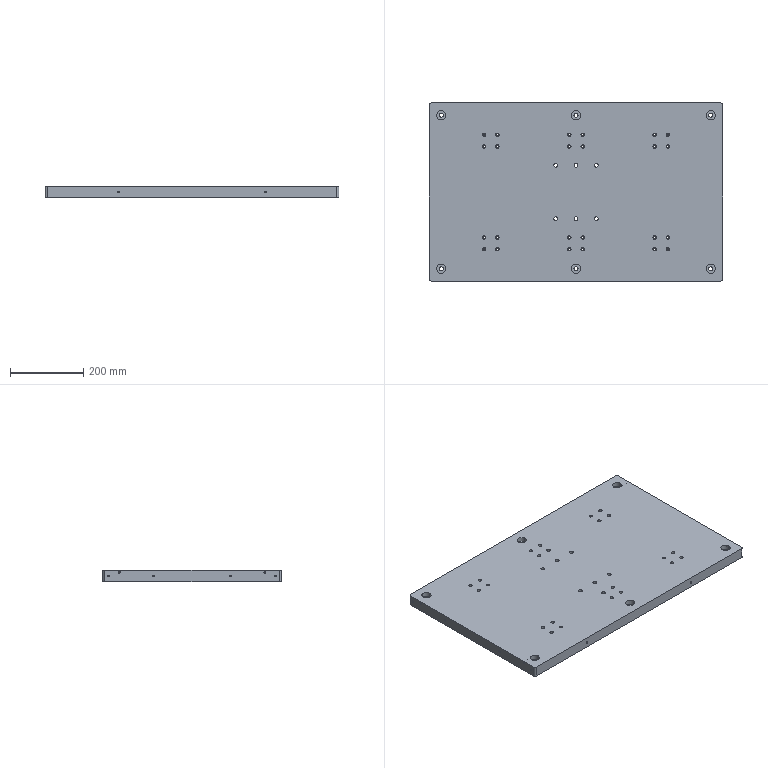Part | 1 solid | 238 faces | box 800 x 485 x 30 mm | volume 11530957 mm3 | cylinder 180 | plane 58 | commonest cylinder face diameters 5.5 x48 9 x48 5.2 x24 10.5 x12 11 x12 16 x12